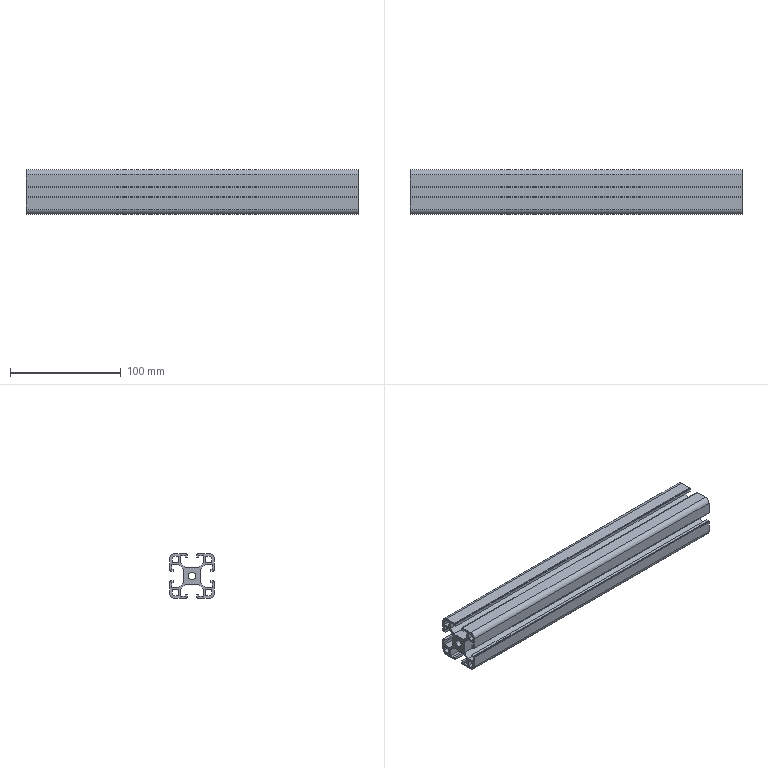Part | SolidWorks | features WeldMemberFeat 1, WeldmentFeature 1 | 1 solid | 104 faces | box 300 x 40 x 40 mm | volume 172964 mm3 | plane 94 | cylinder 10 | commonest cylinder face diameters 5 x4 9 x4 6.8 x2